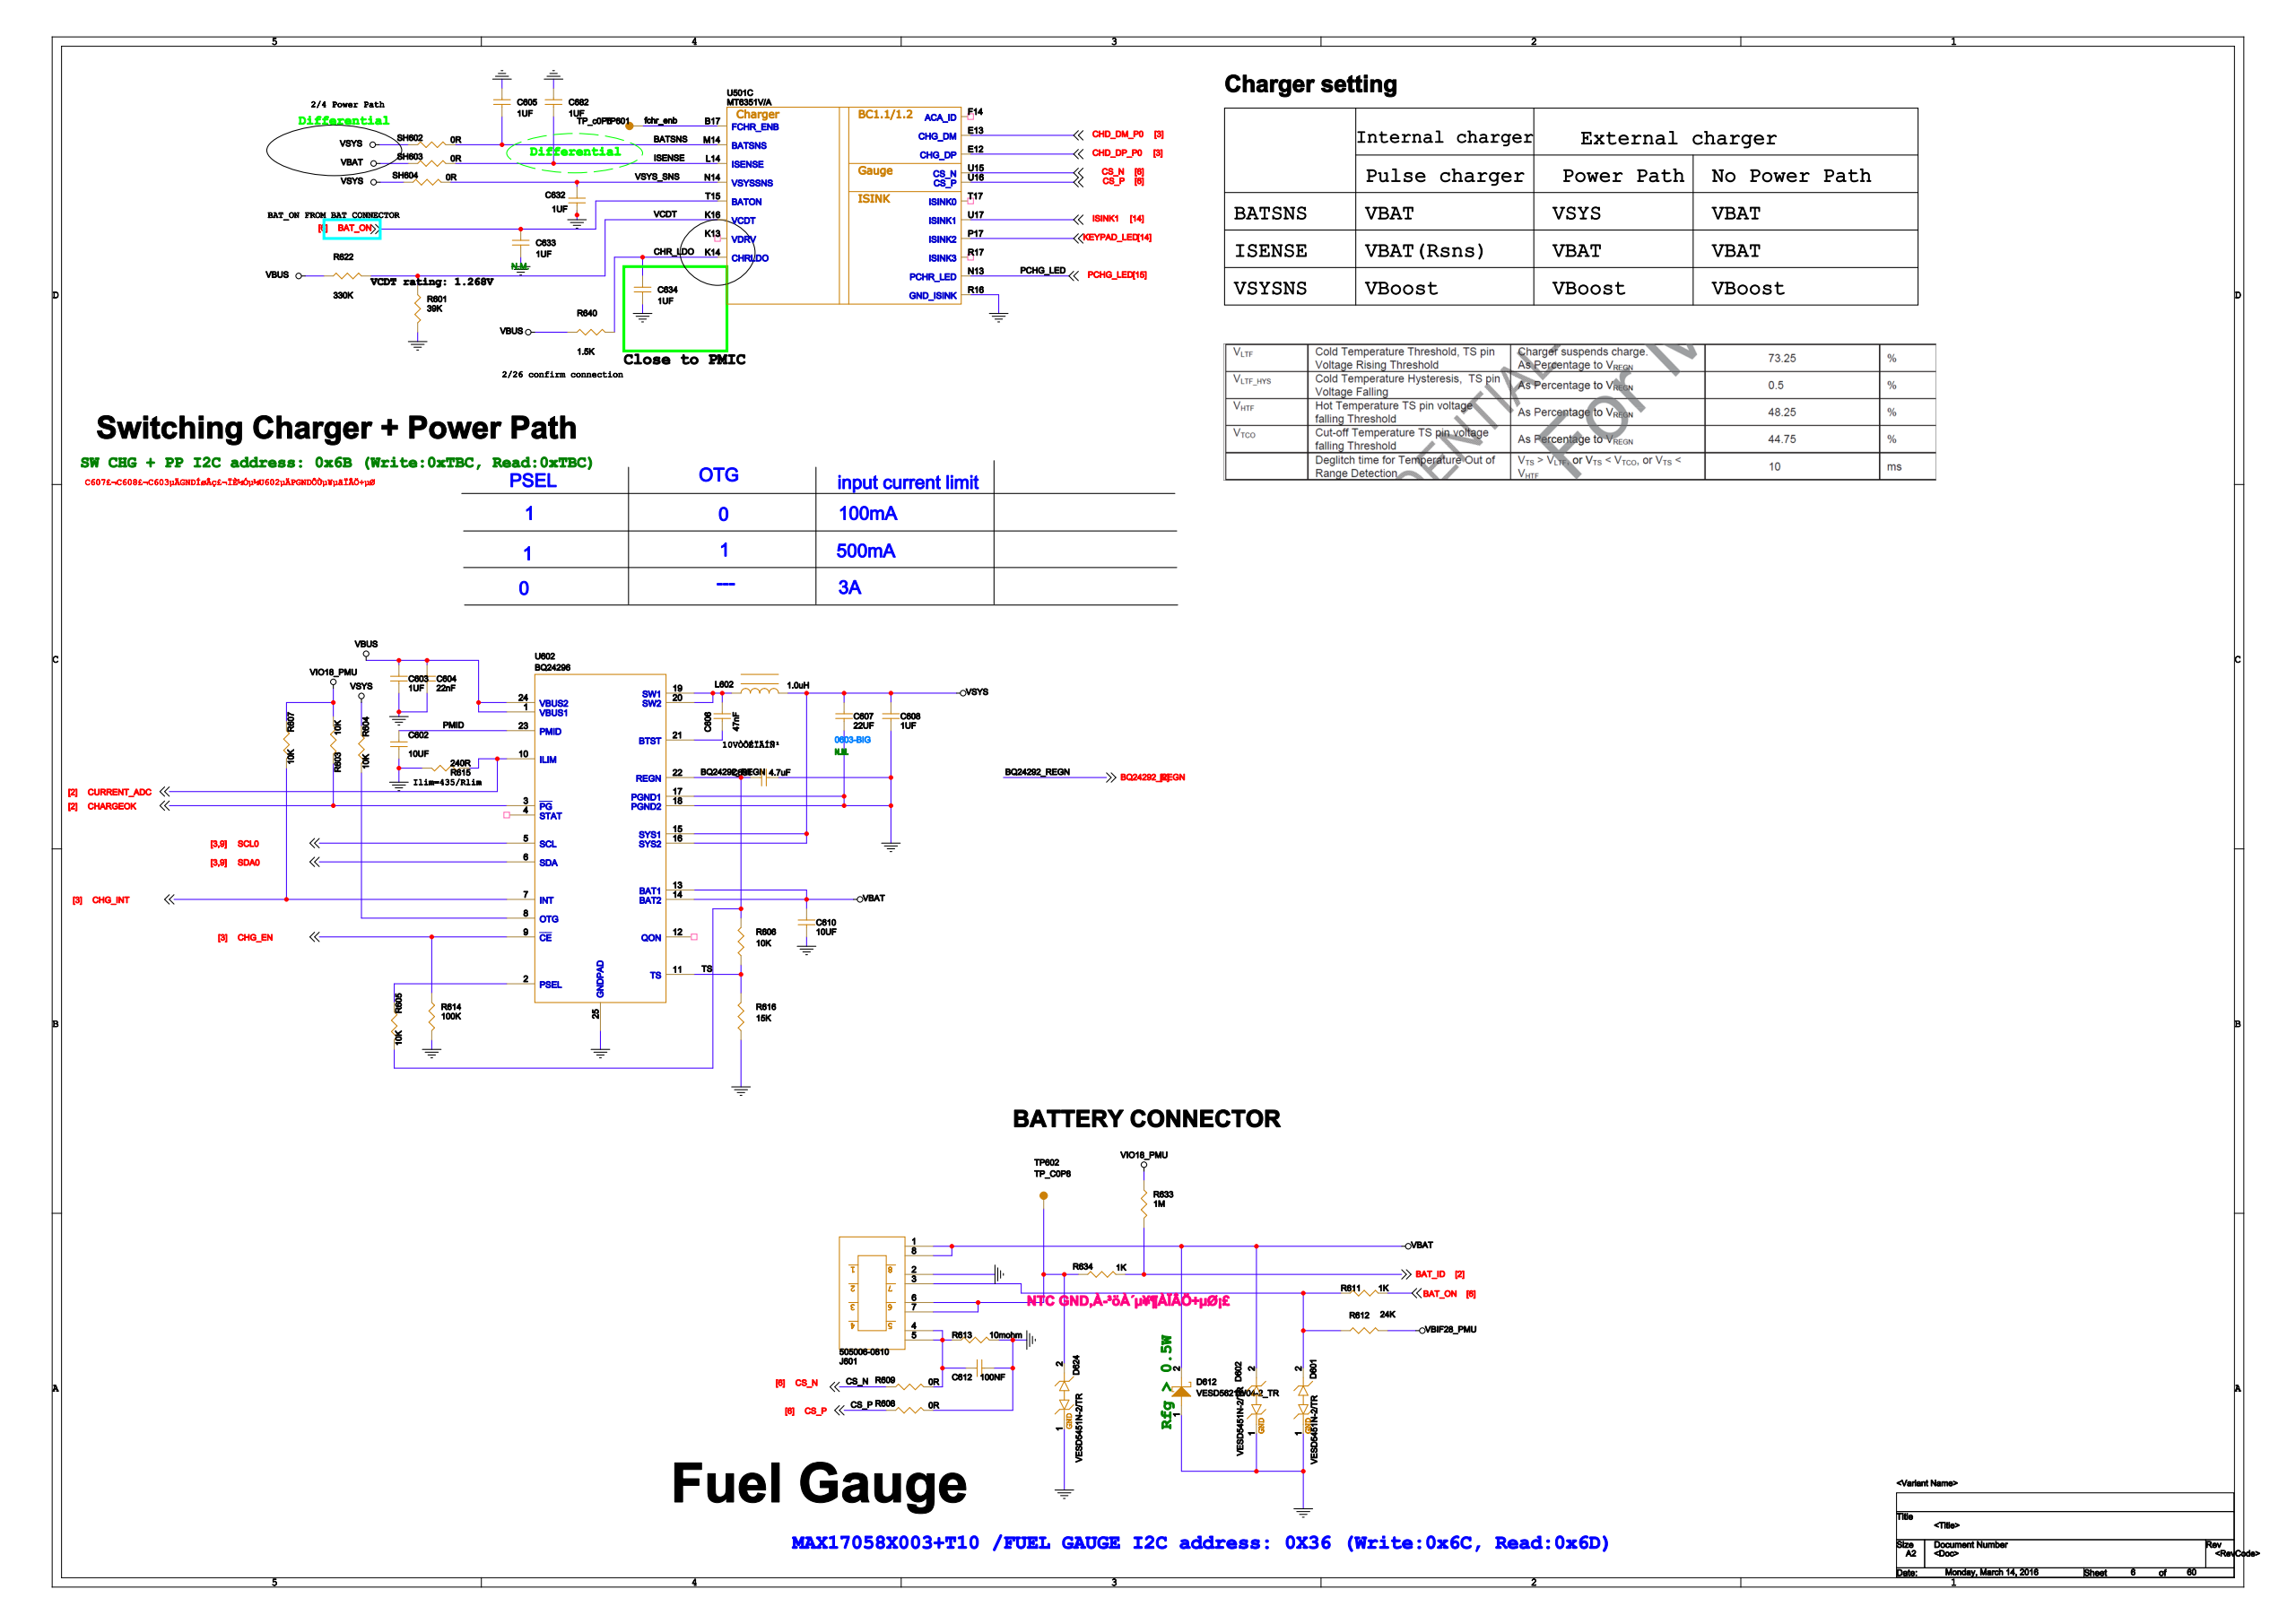Circuit board | Cadence Allegro | 1088 parts | 793 nets | one sheet of the schematic
Parts on this sheet (reference | value | footprint):
C601 | 4.7uF | 0402-BIG
C602 | 10UF | 0402-BIG
C603 | 1UF | C0201
C604 | 22nF | C0201
C605 | 1UF | C0201
C606 | 47nF | C0201
C607
C608 | 1UF | C0201
C610 | 10UF | 0402-BIG
C612 | 100NF | C0201
C632 | 1UF | C0201
C633
C634 | 1UF | C0201
C682 | 1UF | C0201
D601 | VESD5451N-2/TR | DFN1006-2
D602 | VESD5451N-2/TR | DFN1006-2
D612 | VESD5621W04-2_TR | SOD-323F
D624 | VESD5451N-2/TR | DFN1006-2
J601 | 505006-0810 | PWC_SD-505006-001
L602 | 1.0uH | L2520_VLS252010HBX
R601 | 39K | R0201
R603 | 10K | R0201
R604 | 10K | R0201
R605 | 10K | R0201
R606 | 10K | R0201
R607 | 10K | R0201
R608 | 0R | R0201
R609 | 0R | R0201
R611 | 1K | R0201
R612 | 24K | R0201
R613 | 10mohm | R1206_PE1206FKE470R01Z
R614 | 100K | R0201
R615 | 240R | R0201
R616 | 15K | R0201
R622 | 330K | R0201
R633 | 1M | R0201
R634 | 1K | R0201
R640 | 1.5K | R0201
SH602 | 0R | R0201
SH603 | 0R | R0201
SH604 | 0R | R0201
TP602 | TP_C0P8 | TP_C0P8
U501 | MT6351V/A | MT6351
U602 | BQ24296 | QFN24_4X4X1P1_0P5
Nets of these parts (net: part-pin ...):
GND: C601-2 C602-2 C603-2 C604-2 C605-1 C607-2 C608-2 C610-2 C612-2 C632-2 C633-2 C634-2 C682-1 D601-1 D602-1 D612-1 D624-1 J601-2 R601-2 R608-2 R613-2 R614-2 R615-2 R616-1 U501-R16 U602-17 U602-18 U602-25
VBAT: C610-1 D602-2 D612-2 J601-1 J601-8 SH603-1 U602-13 U602-14
VSYS: C607-1 C608-1 L602-2 R604-1 SH602-1 SH604-1 U602-15 U602-16
BAT_ID: R633-2 R634-2
CURRENT_ADC: R615-1 U602-10
CHARGEOK: R603-1 U602-3
CHD_DM_P0: U501-E13
CHD_DP_P0: U501-E12
CHG_INT: R607-2 U602-7
CHG_EN: R614-1 U602-9
SCL0: U602-5
SDA0: U602-6
VIO18_PMU: R603-2 R607-1 R633-1
VBUS: C603-1 C604-1 R622-1 R640-1 U602-1 U602-24
N30702998: C606-1 L602-1 U602-19 U602-20
N30691508: D601-2 J601-3 R611-1 R612-1
N30691577: D624-2 J601-6 J601-7 R634-1 TP602-1
VBIF28_PMU: R612-2
BATSNS: C605-2 SH602-2 U501-M14
VSYS_SNS: C632-1 SH604-2 U501-N14
BAT_ON: C633-1 R611-2 U501-T15
CHR_LDO: C634-1 R640-2 U501-K14
ISENSE: C682-2 SH603-2 U501-L14
BQ24292_REGN: C601-1 R605-2 R606-2 U602-22
N30691514: C612-1 J601-4 J601-5 R609-2 R613-1
PMID: C602-1 U602-23
N30702996: C606-2 U602-21
N30703243: R604-2 U602-8
N30703257: R605-1 U602-2
TS: R606-1 R616-2 U602-11
VCDT: R601-1 R622-2 U501-K16
FCHR_ENB: U501-B17
CS_N: R609-1 U501-U15
CS_P: R608-1 U501-U16
ISINK1: U501-U17
PCHG_LED: U501-N13